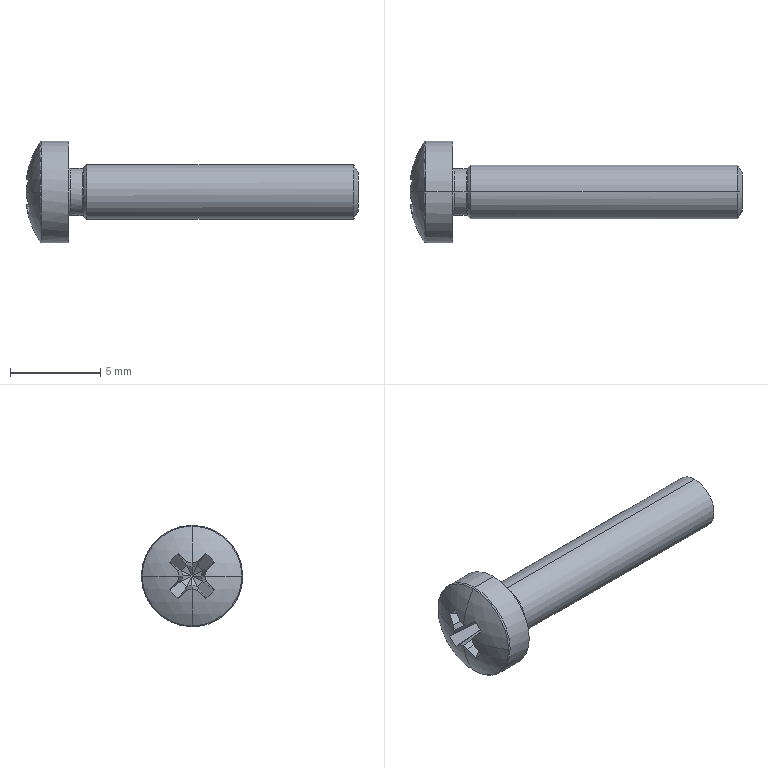Part | STEP file | 103000006242_M3×16 | 1 solid | 54 faces | box 18.351 x 5.6 x 5.6 mm | volume 155.702 mm3 | plane 34 | cylinder 6 | torus 6 | cone 4 | sphere 4 | commonest cylinder face diameters 2.598 x2 3 x2 5.6 x2
STEP:
#1=CARTESIAN_POINT('',(18.4,0.,1.067));
#2=VERTEX_POINT('',#1);
#3=CARTESIAN_POINT('',(18.4,0.,-1.067));
#4=VERTEX_POINT('',#3);
#5=CARTESIAN_POINT('',(18.4,0.,0.));
#6=DIRECTION('',(-1.,0.,0.));
#7=AXIS2_PLACEMENT_3D('',#5,#6,$);
#8=CIRCLE('',#7,1.067);
#9=EDGE_CURVE('',#2,#4,#8,.T.);
#10=ORIENTED_EDGE('',*,*,#9,.T.);
#11=CARTESIAN_POINT('',(18.153,0.,-1.5));
#12=VERTEX_POINT('',#11);
#13=CARTESIAN_POINT('',(-247947.644,0.,-434181.301));
#14=DIRECTION('',(-0.4959,0.,-0.8684));
#15=VECTOR('',#14,1.);
#16=LINE('',#13,#15);
#17=EDGE_CURVE('',#4,#12,#16,.T.);
#18=ORIENTED_EDGE('',*,*,#17,.T.);
#19=CARTESIAN_POINT('',(18.153,0.,1.5));
#20=VERTEX_POINT('',#19);
#21=CARTESIAN_POINT('',(18.153,0.,0.));
#22=DIRECTION('',(-1.,0.,0.));
#23=AXIS2_PLACEMENT_3D('',#21,#22,$);
#24=CIRCLE('',#23,1.5);
#25=EDGE_CURVE('',#20,#12,#24,.T.);
#26=ORIENTED_EDGE('',*,*,#25,.F.);
#27=CARTESIAN_POINT('',(-247947.644,0.,434181.301));
#28=DIRECTION('',(-0.4959,0.,0.8684));
#29=VECTOR('',#28,1.);
#30=LINE('',#27,#29);
#31=EDGE_CURVE('',#2,#20,#30,.T.);
#32=ORIENTED_EDGE('',*,*,#31,.F.);
#33=EDGE_LOOP('',(#10,#18,#26,#32));
#34=FACE_OUTER_BOUND('',#33,.T.);
#35=CARTESIAN_POINT('',(18.153,0.,0.));
#36=DIRECTION('',(-1.,0.,0.));
#37=DIRECTION('',(0.,0.,1.));
#38=AXIS2_PLACEMENT_3D('',#35,#36,#37);
#39=CONICAL_SURFACE('',#38,1.5,1.052);
#40=ADVANCED_FACE('',(#34),#39,.T.);
#41=ORIENTED_EDGE('',*,*,#9,.F.);
#42=CARTESIAN_POINT('',(18.4,0.,0.));
#43=DIRECTION('',(-1.,0.,0.));
#44=AXIS2_PLACEMENT_3D('',#42,#43,$);
#45=CIRCLE('',#44,1.067);
#46=EDGE_CURVE('',#4,#2,#45,.T.);
#47=ORIENTED_EDGE('',*,*,#46,.F.);
#48=EDGE_LOOP('',(#41,#47));
#49=FACE_OUTER_BOUND('',#48,.T.);
#50=CARTESIAN_POINT('',(18.4,0.,0.));
#51=DIRECTION('',(-1.,0.,0.));
#52=DIRECTION('',(0.,0.,1.));
#53=AXIS2_PLACEMENT_3D('',#50,#51,#52);
#54=PLANE('',#53);
#55=ADVANCED_FACE('',(#49),#54,.F.);
#56=ORIENTED_EDGE('',*,*,#17,.F.);
#57=ORIENTED_EDGE('',*,*,#46,.T.);
#58=ORIENTED_EDGE('',*,*,#31,.T.);
#59=CARTESIAN_POINT('',(18.153,0.,0.));
#60=DIRECTION('',(-1.,0.,0.));
#61=AXIS2_PLACEMENT_3D('',#59,#60,$);
#62=CIRCLE('',#61,1.5);
#63=EDGE_CURVE('',#12,#20,#62,.T.);
#64=ORIENTED_EDGE('',*,*,#63,.F.);
#65=EDGE_LOOP('',(#56,#57,#58,#64));
#66=FACE_OUTER_BOUND('',#65,.T.);
#67=CARTESIAN_POINT('',(18.153,0.,0.));
#68=DIRECTION('',(-1.,0.,0.));
#69=DIRECTION('',(0.,0.,-1.));
#70=AXIS2_PLACEMENT_3D('',#67,#68,#69);
#71=CONICAL_SURFACE('',#70,1.5,1.052);
#72=ADVANCED_FACE('',(#66),#71,.T.);
#73=ORIENTED_EDGE('',*,*,#25,.T.);
#74=CARTESIAN_POINT('',(3.4,0.,-1.5));
#75=VERTEX_POINT('',#74);
#76=CARTESIAN_POINT('',(-3.442,0.,-1.5));
#77=DIRECTION('',(-1.,0.,0.));
#78=VECTOR('',#77,1.);
#79=LINE('',#76,#78);
#80=EDGE_CURVE('',#12,#75,#79,.T.);
#81=ORIENTED_EDGE('',*,*,#80,.T.);
#82=CARTESIAN_POINT('',(3.4,0.,1.5));
#83=VERTEX_POINT('',#82);
#84=CARTESIAN_POINT('',(3.4,0.,0.));
#85=DIRECTION('',(-1.,0.,0.));
#86=AXIS2_PLACEMENT_3D('',#84,#85,$);
#87=CIRCLE('',#86,1.5);
#88=EDGE_CURVE('',#83,#75,#87,.T.);
#89=ORIENTED_EDGE('',*,*,#88,.F.);
#90=CARTESIAN_POINT('',(-3.442,0.,1.5));
#91=DIRECTION('',(-1.,0.,0.));
#92=VECTOR('',#91,1.);
#93=LINE('',#90,#92);
#94=EDGE_CURVE('',#20,#83,#93,.T.);
#95=ORIENTED_EDGE('',*,*,#94,.F.);
#96=EDGE_LOOP('',(#73,#81,#89,#95));
#97=FACE_OUTER_BOUND('',#96,.T.);
#98=CARTESIAN_POINT('',(-3.442,0.,0.));
#99=DIRECTION('',(-1.,0.,0.));
#100=DIRECTION('',(0.,0.,1.));
#101=AXIS2_PLACEMENT_3D('',#98,#99,#100);
#102=CYLINDRICAL_SURFACE('',#101,1.5);
#103=ADVANCED_FACE('',(#97),#102,.T.);
#104=ORIENTED_EDGE('',*,*,#80,.F.);
#105=ORIENTED_EDGE('',*,*,#63,.T.);
#106=ORIENTED_EDGE('',*,*,#94,.T.);
#107=CARTESIAN_POINT('',(3.4,0.,-1.5));
#108=CARTESIAN_POINT('',(3.4,-0.4712,-1.5));
#109=CARTESIAN_POINT('',(3.4,-0.9425,-1.315));
#110=CARTESIAN_POINT('',(3.4,-1.315,-0.9425));
#111=CARTESIAN_POINT('',(3.4,-1.685,0.));
#112=CARTESIAN_POINT('',(3.4,-1.315,0.9425));
#113=CARTESIAN_POINT('',(3.4,-0.9425,1.315));
#114=CARTESIAN_POINT('',(3.4,-0.4712,1.5));
#115=CARTESIAN_POINT('',(3.4,0.,1.5));
#116=B_SPLINE_CURVE_WITH_KNOTS('',5,(#107,#108,#109,#110,#111,#112,#113,#114,#115),.UNSPECIFIED.,.F.,.U.,(6,3,6),(-2.356,0.,2.356),.UNSPECIFIED.);
#117=EDGE_CURVE('',#75,#83,#116,.T.);
#118=ORIENTED_EDGE('',*,*,#117,.F.);
#119=EDGE_LOOP('',(#104,#105,#106,#118));
#120=FACE_OUTER_BOUND('',#119,.T.);
#121=CARTESIAN_POINT('',(-3.442,0.,0.));
#122=DIRECTION('',(-1.,0.,0.));
#123=DIRECTION('',(0.,0.,-1.));
#124=AXIS2_PLACEMENT_3D('',#121,#122,#123);
#125=CYLINDRICAL_SURFACE('',#124,1.5);
#126=ADVANCED_FACE('',(#120),#125,.T.);
#127=CARTESIAN_POINT('',(3.228,0.,-1.328));
#128=VERTEX_POINT('',#127);
#129=CARTESIAN_POINT('',(3.228,0.,1.328));
#130=VERTEX_POINT('',#129);
#131=CARTESIAN_POINT('',(3.228,0.,0.));
#132=DIRECTION('',(1.,0.,0.));
#133=AXIS2_PLACEMENT_3D('',#131,#132,$);
#134=CIRCLE('',#133,1.328);
#135=EDGE_CURVE('',#128,#130,#134,.T.);
#136=ORIENTED_EDGE('',*,*,#135,.T.);
#137=CARTESIAN_POINT('',(353556.041,0.,353554.141));
#138=DIRECTION('',(0.7071,0.,0.7071));
#139=VECTOR('',#138,1.);
#140=LINE('',#137,#139);
#141=EDGE_CURVE('',#130,#83,#140,.T.);
#142=ORIENTED_EDGE('',*,*,#141,.T.);
#143=ORIENTED_EDGE('',*,*,#88,.T.);
#144=CARTESIAN_POINT('',(353556.041,0.,-353554.141));
#145=DIRECTION('',(0.7071,0.,-0.7071));
#146=VECTOR('',#145,1.);
#147=LINE('',#144,#146);
#148=EDGE_CURVE('',#128,#75,#147,.T.);
#149=ORIENTED_EDGE('',*,*,#148,.F.);
#150=EDGE_LOOP('',(#136,#142,#143,#149));
#151=FACE_OUTER_BOUND('',#150,.T.);
#152=CARTESIAN_POINT('',(3.4,0.,0.));
#153=DIRECTION('',(1.,0.,0.));
#154=DIRECTION('',(0.,0.,-1.));
#155=AXIS2_PLACEMENT_3D('',#152,#153,#154);
#156=CONICAL_SURFACE('',#155,1.5,0.7854);
#157=ADVANCED_FACE('',(#151),#156,.T.);
#158=ORIENTED_EDGE('',*,*,#141,.F.);
#159=CARTESIAN_POINT('',(3.228,0.,0.));
#160=DIRECTION('',(1.,0.,0.));
#161=AXIS2_PLACEMENT_3D('',#159,#160,$);
#162=CIRCLE('',#161,1.328);
#163=EDGE_CURVE('',#130,#128,#162,.T.);
#164=ORIENTED_EDGE('',*,*,#163,.T.);
#165=ORIENTED_EDGE('',*,*,#148,.T.);
#166=ORIENTED_EDGE('',*,*,#117,.T.);
#167=EDGE_LOOP('',(#158,#164,#165,#166));
#168=FACE_OUTER_BOUND('',#167,.T.);
#169=CARTESIAN_POINT('',(3.4,0.,0.));
#170=DIRECTION('',(1.,0.,0.));
#171=DIRECTION('',(0.,0.,1.));
#172=AXIS2_PLACEMENT_3D('',#169,#170,#171);
#173=CONICAL_SURFACE('',#172,1.5,0.7854);
#174=ADVANCED_FACE('',(#168),#173,.T.);
#175=CARTESIAN_POINT('',(3.158,0.,-1.299));
#176=VERTEX_POINT('',#175);
#177=CARTESIAN_POINT('',(3.158,0.,-1.399));
#178=DIRECTION('',(0.,1.,0.));
#179=AXIS2_PLACEMENT_3D('',#177,#178,$);
#180=CIRCLE('',#179,0.1);
#181=EDGE_CURVE('',#176,#128,#180,.T.);
#182=ORIENTED_EDGE('',*,*,#181,.F.);
#183=CARTESIAN_POINT('',(3.158,0.,1.299));
#184=VERTEX_POINT('',#183);
#185=CARTESIAN_POINT('',(3.158,0.,0.));
#186=DIRECTION('',(-1.,0.,0.));
#187=AXIS2_PLACEMENT_3D('',#185,#186,$);
#188=CIRCLE('',#187,1.299);
#189=EDGE_CURVE('',#184,#176,#188,.T.);
#190=ORIENTED_EDGE('',*,*,#189,.F.);
#191=CARTESIAN_POINT('',(3.158,0.,1.399));
#192=DIRECTION('',(0.,-1.,0.));
#193=AXIS2_PLACEMENT_3D('',#191,#192,$);
#194=CIRCLE('',#193,0.1);
#195=EDGE_CURVE('',#184,#130,#194,.T.);
#196=ORIENTED_EDGE('',*,*,#195,.T.);
#197=ORIENTED_EDGE('',*,*,#135,.F.);
#198=EDGE_LOOP('',(#182,#190,#196,#197));
#199=FACE_OUTER_BOUND('',#198,.T.);
#200=CARTESIAN_POINT('',(3.158,0.,0.));
#201=DIRECTION('',(-1.,0.,0.));
#202=DIRECTION('',(0.,0.,1.));
#203=AXIS2_PLACEMENT_3D('',#200,#201,#202);
#204=TOROIDAL_SURFACE('',#203,1.399,0.1);
#205=ADVANCED_FACE('',(#199),#204,.F.);
#206=CARTESIAN_POINT('',(3.158,0.,0.));
#207=DIRECTION('',(-1.,0.,0.));
#208=AXIS2_PLACEMENT_3D('',#206,#207,$);
#209=CIRCLE('',#208,1.299);
#210=EDGE_CURVE('',#176,#184,#209,.T.);
#211=ORIENTED_EDGE('',*,*,#210,.F.);
#212=ORIENTED_EDGE('',*,*,#181,.T.);
#213=ORIENTED_EDGE('',*,*,#163,.F.);
#214=ORIENTED_EDGE('',*,*,#195,.F.);
#215=EDGE_LOOP('',(#211,#212,#213,#214));
#216=FACE_OUTER_BOUND('',#215,.T.);
#217=CARTESIAN_POINT('',(3.158,0.,0.));
#218=DIRECTION('',(-1.,0.,0.));
#219=DIRECTION('',(0.,0.,-1.));
#220=AXIS2_PLACEMENT_3D('',#217,#218,#219);
#221=TOROIDAL_SURFACE('',#220,1.399,0.1);
#222=ADVANCED_FACE('',(#216),#221,.F.);
#223=ORIENTED_EDGE('',*,*,#189,.T.);
#224=CARTESIAN_POINT('',(2.5,0.,-1.299));
#225=VERTEX_POINT('',#224);
#226=CARTESIAN_POINT('',(-3.442,0.,-1.299));
#227=DIRECTION('',(-1.,0.,0.));
#228=VECTOR('',#227,1.);
#229=LINE('',#226,#228);
#230=EDGE_CURVE('',#176,#225,#229,.T.);
#231=ORIENTED_EDGE('',*,*,#230,.T.);
#232=CARTESIAN_POINT('',(2.5,0.,1.299));
#233=VERTEX_POINT('',#232);
#234=CARTESIAN_POINT('',(2.5,0.,0.));
#235=DIRECTION('',(-1.,0.,0.));
#236=AXIS2_PLACEMENT_3D('',#234,#235,$);
#237=CIRCLE('',#236,1.299);
#238=EDGE_CURVE('',#225,#233,#237,.F.);
#239=ORIENTED_EDGE('',*,*,#238,.T.);
#240=CARTESIAN_POINT('',(-3.442,0.,1.299));
#241=DIRECTION('',(-1.,0.,0.));
#242=VECTOR('',#241,1.);
#243=LINE('',#240,#242);
#244=EDGE_CURVE('',#184,#233,#243,.T.);
#245=ORIENTED_EDGE('',*,*,#244,.F.);
#246=EDGE_LOOP('',(#223,#231,#239,#245));
#247=FACE_OUTER_BOUND('',#246,.T.);
#248=CARTESIAN_POINT('',(-3.442,0.,0.));
#249=DIRECTION('',(-1.,0.,0.));
#250=DIRECTION('',(0.,0.,1.));
#251=AXIS2_PLACEMENT_3D('',#248,#249,#250);
#252=CYLINDRICAL_SURFACE('',#251,1.299);
#253=ADVANCED_FACE('',(#247),#252,.T.);
#254=ORIENTED_EDGE('',*,*,#230,.F.);
#255=ORIENTED_EDGE('',*,*,#210,.T.);
#256=ORIENTED_EDGE('',*,*,#244,.T.);
#257=CARTESIAN_POINT('',(2.5,0.,1.299));
#258=CARTESIAN_POINT('',(2.5,-0.4081,1.299));
#259=CARTESIAN_POINT('',(2.5,-0.8162,1.139));
#260=CARTESIAN_POINT('',(2.5,-1.139,0.8162));
#261=CARTESIAN_POINT('',(2.5,-1.459,0.));
#262=CARTESIAN_POINT('',(2.5,-1.139,-0.8162));
#263=CARTESIAN_POINT('',(2.5,-0.8162,-1.139));
#264=CARTESIAN_POINT('',(2.5,-0.4081,-1.299));
#265=CARTESIAN_POINT('',(2.5,0.,-1.299));
#266=B_SPLINE_CURVE_WITH_KNOTS('',5,(#257,#258,#259,#260,#261,#262,#263,#264,#265),.UNSPECIFIED.,.F.,.U.,(6,3,6),(-2.04,0.,2.04),.UNSPECIFIED.);
#267=EDGE_CURVE('',#233,#225,#266,.T.);
#268=ORIENTED_EDGE('',*,*,#267,.T.);
#269=EDGE_LOOP('',(#254,#255,#256,#268));
#270=FACE_OUTER_BOUND('',#269,.T.);
#271=CARTESIAN_POINT('',(-3.442,0.,0.));
#272=DIRECTION('',(-1.,0.,0.));
#273=DIRECTION('',(0.,0.,-1.));
#274=AXIS2_PLACEMENT_3D('',#271,#272,#273);
#275=CYLINDRICAL_SURFACE('',#274,1.299);
#276=ADVANCED_FACE('',(#270),#275,.T.);
#277=CARTESIAN_POINT('',(2.4,0.,-1.399));
#278=VERTEX_POINT('',#277);
#279=CARTESIAN_POINT('',(2.5,0.,-1.399));
#280=DIRECTION('',(0.,1.,0.));
#281=AXIS2_PLACEMENT_3D('',#279,#280,$);
#282=CIRCLE('',#281,0.1);
#283=EDGE_CURVE('',#278,#225,#282,.T.);
#284=ORIENTED_EDGE('',*,*,#283,.F.);
#285=CARTESIAN_POINT('',(2.4,0.,1.399));
#286=VERTEX_POINT('',#285);
#287=CARTESIAN_POINT('',(2.4,0.,0.));
#288=DIRECTION('',(-1.,0.,0.));
#289=AXIS2_PLACEMENT_3D('',#287,#288,$);
#290=CIRCLE('',#289,1.399);
#291=EDGE_CURVE('',#286,#278,#290,.T.);
#292=ORIENTED_EDGE('',*,*,#291,.F.);
#293=CARTESIAN_POINT('',(2.5,0.,1.399));
#294=DIRECTION('',(0.,-1.,0.));
#295=AXIS2_PLACEMENT_3D('',#293,#294,$);
#296=CIRCLE('',#295,0.1);
#297=EDGE_CURVE('',#286,#233,#296,.T.);
#298=ORIENTED_EDGE('',*,*,#297,.T.);
#299=ORIENTED_EDGE('',*,*,#238,.F.);
#300=EDGE_LOOP('',(#284,#292,#298,#299));
#301=FACE_OUTER_BOUND('',#300,.T.);
#302=CARTESIAN_POINT('',(2.5,0.,0.));
#303=DIRECTION('',(-1.,0.,0.));
#304=DIRECTION('',(0.,0.,1.));
#305=AXIS2_PLACEMENT_3D('',#302,#303,#304);
#306=TOROIDAL_SURFACE('',#305,1.399,0.1);
#307=ADVANCED_FACE('',(#301),#306,.F.);
#308=CARTESIAN_POINT('',(2.4,0.,0.));
#309=DIRECTION('',(-1.,0.,0.));
#310=AXIS2_PLACEMENT_3D('',#308,#309,$);
#311=CIRCLE('',#310,1.399);
#312=EDGE_CURVE('',#278,#286,#311,.T.);
#313=ORIENTED_EDGE('',*,*,#312,.F.);
#314=ORIENTED_EDGE('',*,*,#283,.T.);
#315=ORIENTED_EDGE('',*,*,#267,.F.);
#316=ORIENTED_EDGE('',*,*,#297,.F.);
#317=EDGE_LOOP('',(#313,#314,#315,#316));
#318=FACE_OUTER_BOUND('',#317,.T.);
#319=CARTESIAN_POINT('',(2.5,0.,0.));
#320=DIRECTION('',(-1.,0.,0.));
#321=DIRECTION('',(0.,0.,-1.));
#322=AXIS2_PLACEMENT_3D('',#319,#320,#321);
#323=TOROIDAL_SURFACE('',#322,1.399,0.1);
#324=ADVANCED_FACE('',(#318),#323,.F.);
#325=CARTESIAN_POINT('',(2.4,0.,2.8));
#326=VERTEX_POINT('',#325);
#327=CARTESIAN_POINT('',(2.4,0.,-2.8));
#328=VERTEX_POINT('',#327);
#329=CARTESIAN_POINT('',(2.4,-0.000000001,0.));
#330=DIRECTION('',(-1.,0.,0.));
#331=AXIS2_PLACEMENT_3D('',#329,#330,$);
#332=CIRCLE('',#331,2.8);
#333=EDGE_CURVE('',#326,#328,#332,.T.);
#334=ORIENTED_EDGE('',*,*,#333,.F.);
#335=CARTESIAN_POINT('',(2.4,0.000000001,0.));
#336=DIRECTION('',(-1.,0.,0.));
#337=AXIS2_PLACEMENT_3D('',#335,#336,$);
#338=CIRCLE('',#337,2.8);
#339=EDGE_CURVE('',#328,#326,#338,.T.);
#340=ORIENTED_EDGE('',*,*,#339,.F.);
#341=EDGE_LOOP('',(#334,#340));
#342=FACE_OUTER_BOUND('',#341,.T.);
#343=ORIENTED_EDGE('',*,*,#291,.T.);
#344=ORIENTED_EDGE('',*,*,#312,.T.);
#345=EDGE_LOOP('',(#343,#344));
#346=FACE_BOUND('',#345,.T.);
#347=CARTESIAN_POINT('',(2.4,2.8,0.));
#348=DIRECTION('',(-1.,0.,0.));
#349=DIRECTION('',(0.,0.,1.));
#350=AXIS2_PLACEMENT_3D('',#347,#348,#349);
#351=PLANE('',#350);
#352=ADVANCED_FACE('',(#342,#346),#351,.F.);
#353=ORIENTED_EDGE('',*,*,#333,.T.);
#354=CARTESIAN_POINT('',(0.911,0.,-2.8));
#355=VERTEX_POINT('',#354);
#356=CARTESIAN_POINT('',(-3.442,0.,-2.8));
#357=DIRECTION('',(-1.,0.,0.));
#358=VECTOR('',#357,1.);
#359=LINE('',#356,#358);
#360=EDGE_CURVE('',#328,#355,#359,.T.);
#361=ORIENTED_EDGE('',*,*,#360,.T.);
#362=CARTESIAN_POINT('',(0.911,0.,2.8));
#363=VERTEX_POINT('',#362);
#364=CARTESIAN_POINT('',(0.911,0.,0.));
#365=DIRECTION('',(-1.,0.,0.));
#366=AXIS2_PLACEMENT_3D('',#364,#365,$);
#367=CIRCLE('',#366,2.8);
#368=EDGE_CURVE('',#355,#363,#367,.F.);
#369=ORIENTED_EDGE('',*,*,#368,.T.);
#370=CARTESIAN_POINT('',(-3.442,0.,2.8));
#371=DIRECTION('',(-1.,0.,0.));
#372=VECTOR('',#371,1.);
#373=LINE('',#370,#372);
#374=EDGE_CURVE('',#326,#363,#373,.T.);
#375=ORIENTED_EDGE('',*,*,#374,.F.);
#376=EDGE_LOOP('',(#353,#361,#369,#375));
#377=FACE_OUTER_BOUND('',#376,.T.);
#378=CARTESIAN_POINT('',(-3.442,0.,0.));
#379=DIRECTION('',(-1.,0.,0.));
#380=DIRECTION('',(0.,0.,1.));
#381=AXIS2_PLACEMENT_3D('',#378,#379,#380);
#382=CYLINDRICAL_SURFACE('',#381,2.8);
#383=ADVANCED_FACE('',(#377),#382,.T.);
#384=ORIENTED_EDGE('',*,*,#360,.F.);
#385=ORIENTED_EDGE('',*,*,#339,.T.);
#386=ORIENTED_EDGE('',*,*,#374,.T.);
#387=CARTESIAN_POINT('',(0.911,0.,2.8));
#388=CARTESIAN_POINT('',(0.911,-0.8796,2.8));
#389=CARTESIAN_POINT('',(0.911,-1.759,2.455));
#390=CARTESIAN_POINT('',(0.911,-2.455,1.759));
#391=CARTESIAN_POINT('',(0.911,-3.145,0.));
#392=CARTESIAN_POINT('',(0.911,-2.455,-1.759));
#393=CARTESIAN_POINT('',(0.911,-1.759,-2.455));
#394=CARTESIAN_POINT('',(0.911,-0.8796,-2.8));
#395=CARTESIAN_POINT('',(0.911,0.,-2.8));
#396=B_SPLINE_CURVE_WITH_KNOTS('',5,(#387,#388,#389,#390,#391,#392,#393,#394,#395),.UNSPECIFIED.,.F.,.U.,(6,3,6),(-4.398,0.,4.398),.UNSPECIFIED.);
#397=EDGE_CURVE('',#363,#355,#396,.T.);
#398=ORIENTED_EDGE('',*,*,#397,.T.);
#399=EDGE_LOOP('',(#384,#385,#386,#398));
#400=FACE_OUTER_BOUND('',#399,.T.);
#401=CARTESIAN_POINT('',(-3.442,0.,0.));
#402=DIRECTION('',(-1.,0.,0.));
#403=DIRECTION('',(0.,0.,-1.));
#404=AXIS2_PLACEMENT_3D('',#401,#402,#403);
#405=CYLINDRICAL_SURFACE('',#404,2.8);
#406=ADVANCED_FACE('',(#400),#405,.T.);
#407=CARTESIAN_POINT('',(0.8275,0.,2.755));
#408=VERTEX_POINT('',#407);
#409=CARTESIAN_POINT('',(0.8275,2.755,0.));
#410=VERTEX_POINT('',#409);
#411=CARTESIAN_POINT('',(0.8275,0.,0.));
#412=DIRECTION('',(1.,0.,0.));
#413=AXIS2_PLACEMENT_3D('',#411,#412,$);
#414=CIRCLE('',#413,2.755);
#415=EDGE_CURVE('',#408,#410,#414,.F.);
#416=ORIENTED_EDGE('',*,*,#415,.F.);
#417=CARTESIAN_POINT('',(0.911,0.,2.7));
#418=DIRECTION('',(0.,1.,0.));
#419=AXIS2_PLACEMENT_3D('',#417,#418,$);
#420=CIRCLE('',#419,0.1);
#421=EDGE_CURVE('',#408,#363,#420,.T.);
#422=ORIENTED_EDGE('',*,*,#421,.T.);
#423=ORIENTED_EDGE('',*,*,#368,.F.);
#424=CARTESIAN_POINT('',(0.8275,0.,-2.755));
#425=VERTEX_POINT('',#424);
#426=CARTESIAN_POINT('',(0.911,0.,-2.7));
#427=DIRECTION('',(0.,-1.,0.));
#428=AXIS2_PLACEMENT_3D('',#426,#427,$);
#429=CIRCLE('',#428,0.1);
#430=EDGE_CURVE('',#425,#355,#429,.T.);
#431=ORIENTED_EDGE('',*,*,#430,.F.);
#432=CARTESIAN_POINT('',(0.8275,0.,0.));
#433=DIRECTION('',(1.,0.,0.));
#434=AXIS2_PLACEMENT_3D('',#432,#433,$);
#435=CIRCLE('',#434,2.755);
#436=EDGE_CURVE('',#410,#425,#435,.F.);
#437=ORIENTED_EDGE('',*,*,#436,.F.);
#438=EDGE_LOOP('',(#416,#422,#423,#431,#437));
#439=FACE_OUTER_BOUND('',#438,.T.);
#440=CARTESIAN_POINT('',(0.911,0.,0.));
#441=DIRECTION('',(1.,0.,0.));
#442=DIRECTION('',(0.,0.,-1.));
#443=AXIS2_PLACEMENT_3D('',#440,#441,#442);
#444=TOROIDAL_SURFACE('',#443,2.7,0.1);
#445=ADVANCED_FACE('',(#439),#444,.T.);
#446=ORIENTED_EDGE('',*,*,#421,.F.);
#447=CARTESIAN_POINT('',(0.8275,-2.755,0.));
#448=VERTEX_POINT('',#447);
#449=CARTESIAN_POINT('',(0.8275,0.,0.));
#450=DIRECTION('',(1.,0.,0.));
#451=AXIS2_PLACEMENT_3D('',#449,#450,$);
#452=CIRCLE('',#451,2.755);
#453=EDGE_CURVE('',#448,#408,#452,.F.);
#454=ORIENTED_EDGE('',*,*,#453,.F.);
#455=CARTESIAN_POINT('',(0.8275,0.,0.));
#456=DIRECTION('',(1.,0.,0.));
#457=AXIS2_PLACEMENT_3D('',#455,#456,$);
#458=CIRCLE('',#457,2.755);
#459=EDGE_CURVE('',#425,#448,#458,.F.);
#460=ORIENTED_EDGE('',*,*,#459,.F.);
#461=ORIENTED_EDGE('',*,*,#430,.T.);
#462=ORIENTED_EDGE('',*,*,#397,.F.);
#463=EDGE_LOOP('',(#446,#454,#460,#461,#462));
#464=FACE_OUTER_BOUND('',#463,.T.);
#465=CARTESIAN_POINT('',(0.911,0.,0.));
#466=DIRECTION('',(1.,0.,0.));
#467=DIRECTION('',(0.,0.,1.));
#468=AXIS2_PLACEMENT_3D('',#465,#466,#467);
#469=TOROIDAL_SURFACE('',#468,2.7,0.1);
#470=ADVANCED_FACE('',(#464),#469,.T.);
#471=CARTESIAN_POINT('',(0.04924,0.,0.7));
#472=VERTEX_POINT('',#471);
#473=CARTESIAN_POINT('',(5.,0.,0.));
#474=DIRECTION('',(0.,-1.,0.));
#475=AXIS2_PLACEMENT_3D('',#473,#474,$);
#476=CIRCLE('',#475,5.);
#477=EDGE_CURVE('',#408,#472,#476,.T.);
#478=ORIENTED_EDGE('',*,*,#477,.F.);
#479=ORIENTED_EDGE('',*,*,#415,.T.);
#480=CARTESIAN_POINT('',(0.04924,0.7,0.));
#481=VERTEX_POINT('',#480);
#482=CARTESIAN_POINT('',(5.,0.,0.));
#483=DIRECTION('',(0.,0.,-1.));
#484=AXIS2_PLACEMENT_3D('',#482,#483,$);
#485=CIRCLE('',#484,5.);
#486=EDGE_CURVE('',#410,#481,#485,.F.);
#487=ORIENTED_EDGE('',*,*,#486,.T.);
#488=CARTESIAN_POINT('',(0.0753,0.8113,0.2985));
#489=VERTEX_POINT('',#488);
#490=CARTESIAN_POINT('',(0.04924,0.7,0.));
#491=CARTESIAN_POINT('',(0.05455,0.7375,0.09958));
#492=CARTESIAN_POINT('',(0.06324,0.7747,0.1991));
#493=CARTESIAN_POINT('',(0.0753,0.8113,0.2985));
#494=B_SPLINE_CURVE_WITH_KNOTS('',3,(#490,#491,#492,#493),.UNSPECIFIED.,.F.,.U.,(4,4),(0.,0.4521),.UNSPECIFIED.);
#495=EDGE_CURVE('',#481,#489,#494,.T.);
#496=ORIENTED_EDGE('',*,*,#495,.T.);
#497=CARTESIAN_POINT('',(0.2189,1.246,0.7669));
#498=VERTEX_POINT('',#497);
#499=CARTESIAN_POINT('',(0.0753,0.8113,0.2985));
#500=CARTESIAN_POINT('',(0.1092,0.9593,0.4559));
#501=CARTESIAN_POINT('',(0.1573,1.105,0.6126));
#502=CARTESIAN_POINT('',(0.2189,1.246,0.7669));
#503=B_SPLINE_CURVE_WITH_KNOTS('',3,(#499,#500,#501,#502),.UNSPECIFIED.,.F.,.U.,(4,4),(0.,0.9283),.UNSPECIFIED.);
#504=EDGE_CURVE('',#489,#498,#503,.T.);
#505=ORIENTED_EDGE('',*,*,#504,.T.);
#506=CARTESIAN_POINT('',(0.2189,0.7669,1.246));
#507=VERTEX_POINT('',#506);
#508=CARTESIAN_POINT('',(0.2189,0.7669,1.246));
#509=CARTESIAN_POINT('',(0.205,0.9307,1.092));
#510=CARTESIAN_POINT('',(0.2049,1.091,0.9316));
#511=CARTESIAN_POINT('',(0.2189,1.246,0.7669));
#512=B_SPLINE_CURVE_WITH_KNOTS('',3,(#508,#509,#510,#511),.UNSPECIFIED.,.F.,.U.,(4,4),(0.,0.9641),.UNSPECIFIED.);
#513=EDGE_CURVE('',#507,#498,#512,.T.);
#514=ORIENTED_EDGE('',*,*,#513,.F.);
#515=CARTESIAN_POINT('',(0.0753,0.2985,0.8113));
#516=VERTEX_POINT('',#515);
#517=CARTESIAN_POINT('',(0.2189,0.7669,1.246));
#518=CARTESIAN_POINT('',(0.1574,0.6128,1.105));
#519=CARTESIAN_POINT('',(0.1093,0.4562,0.9595));
#520=CARTESIAN_POINT('',(0.0753,0.2985,0.8113));
#521=B_SPLINE_CURVE_WITH_KNOTS('',3,(#517,#518,#519,#520),.UNSPECIFIED.,.F.,.U.,(4,4),(0.,0.9325),.UNSPECIFIED.);
#522=EDGE_CURVE('',#507,#516,#521,.T.);
#523=ORIENTED_EDGE('',*,*,#522,.T.);
#524=CARTESIAN_POINT('',(0.0753,0.2985,0.8113));
#525=CARTESIAN_POINT('',(0.06325,0.1992,0.7747));
#526=CARTESIAN_POINT('',(0.05455,0.09965,0.7376));
#527=CARTESIAN_POINT('',(0.04924,0.,0.7));
#528=B_SPLINE_CURVE_WITH_KNOTS('',3,(#524,#525,#526,#527),.UNSPECIFIED.,.F.,.U.,(4,4),(0.,0.4544),.UNSPECIFIED.);
#529=EDGE_CURVE('',#516,#472,#528,.T.);
#530=ORIENTED_EDGE('',*,*,#529,.T.);
#531=EDGE_LOOP('',(#478,#479,#487,#496,#505,#514,#523,#530));
#532=FACE_OUTER_BOUND('',#531,.T.);
#533=CARTESIAN_POINT('',(5.,0.,0.));
#534=DIRECTION('',(0.,0.,-1.));
#535=DIRECTION('',(-1.,0.,0.));
#536=AXIS2_PLACEMENT_3D('',#533,#534,#535);
#537=SPHERICAL_SURFACE('',#536,5.);
#538=ADVANCED_FACE('',(#532),#537,.T.);
#539=CARTESIAN_POINT('',(0.04924,0.,-0.7));
#540=VERTEX_POINT('',#539);
#541=CARTESIAN_POINT('',(5.,0.,0.));
#542=DIRECTION('',(0.,-1.,0.));
#543=AXIS2_PLACEMENT_3D('',#541,#542,$);
#544=CIRCLE('',#543,5.);
#545=EDGE_CURVE('',#540,#425,#544,.T.);
#546=ORIENTED_EDGE('',*,*,#545,.F.);
#547=CARTESIAN_POINT('',(0.0753,0.2985,-0.8113));
#548=VERTEX_POINT('',#547);
#549=CARTESIAN_POINT('',(0.04924,0.,-0.7));
#550=CARTESIAN_POINT('',(0.05455,0.09965,-0.7376));
#551=CARTESIAN_POINT('',(0.06325,0.1992,-0.7747));
#552=CARTESIAN_POINT('',(0.0753,0.2985,-0.8113));
#553=B_SPLINE_CURVE_WITH_KNOTS('',3,(#549,#550,#551,#552),.UNSPECIFIED.,.F.,.U.,(4,4),(0.,0.4544),.UNSPECIFIED.);
#554=EDGE_CURVE('',#540,#548,#553,.T.);
#555=ORIENTED_EDGE('',*,*,#554,.T.);
#556=CARTESIAN_POINT('',(0.2189,0.7669,-1.246));
#557=VERTEX_POINT('',#556);
#558=CARTESIAN_POINT('',(0.0753,0.2985,-0.8113));
#559=CARTESIAN_POINT('',(0.1093,0.4562,-0.9595));
#560=CARTESIAN_POINT('',(0.1574,0.6128,-1.105));
#561=CARTESIAN_POINT('',(0.2189,0.7669,-1.246));
#562=B_SPLINE_CURVE_WITH_KNOTS('',3,(#558,#559,#560,#561),.UNSPECIFIED.,.F.,.U.,(4,4),(0.,0.9325),.UNSPECIFIED.);
#563=EDGE_CURVE('',#548,#557,#562,.T.);
#564=ORIENTED_EDGE('',*,*,#563,.T.);
#565=CARTESIAN_POINT('',(0.2189,1.246,-0.7669));
#566=VERTEX_POINT('',#565);
#567=CARTESIAN_POINT('',(0.2189,1.246,-0.7669));
#568=CARTESIAN_POINT('',(0.2049,1.091,-0.9316));
#569=CARTESIAN_POINT('',(0.205,0.9307,-1.092));
#570=CARTESIAN_POINT('',(0.2189,0.7669,-1.246));
#571=B_SPLINE_CURVE_WITH_KNOTS('',3,(#567,#568,#569,#570),.UNSPECIFIED.,.F.,.U.,(4,4),(0.,0.9641),.UNSPECIFIED.);
#572=EDGE_CURVE('',#566,#557,#571,.T.);
#573=ORIENTED_EDGE('',*,*,#572,.F.);
#574=CARTESIAN_POINT('',(0.0753,0.8113,-0.2985));
#575=VERTEX_POINT('',#574);
#576=CARTESIAN_POINT('',(0.2189,1.246,-0.7669));
#577=CARTESIAN_POINT('',(0.1573,1.105,-0.6126));
#578=CARTESIAN_POINT('',(0.1092,0.9593,-0.4559));
#579=CARTESIAN_POINT('',(0.0753,0.8113,-0.2985));
#580=B_SPLINE_CURVE_WITH_KNOTS('',3,(#576,#577,#578,#579),.UNSPECIFIED.,.F.,.U.,(4,4),(0.,0.9283),.UNSPECIFIED.);
#581=EDGE_CURVE('',#566,#575,#580,.T.);
#582=ORIENTED_EDGE('',*,*,#581,.T.);
#583=CARTESIAN_POINT('',(0.0753,0.8113,-0.2985));
#584=CARTESIAN_POINT('',(0.06324,0.7747,-0.1991));
#585=CARTESIAN_POINT('',(0.05455,0.7375,-0.09958));
#586=CARTESIAN_POINT('',(0.04924,0.7,0.));
#587=B_SPLINE_CURVE_WITH_KNOTS('',3,(#583,#584,#585,#586),.UNSPECIFIED.,.F.,.U.,(4,4),(0.,0.4521),.UNSPECIFIED.);
#588=EDGE_CURVE('',#575,#481,#587,.T.);
#589=ORIENTED_EDGE('',*,*,#588,.T.);
#590=ORIENTED_EDGE('',*,*,#486,.F.);
#591=ORIENTED_EDGE('',*,*,#436,.T.);
#592=EDGE_LOOP('',(#546,#555,#564,#573,#582,#589,#590,#591));
#593=FACE_OUTER_BOUND('',#592,.T.);
#594=CARTESIAN_POINT('',(5.,0.,0.));
#595=DIRECTION('',(0.,0.,-1.));
#596=DIRECTION('',(-1.,0.,0.));
#597=AXIS2_PLACEMENT_3D('',#594,#595,#596);
#598=SPHERICAL_SURFACE('',#597,5.);
#599=ADVANCED_FACE('',(#593),#598,.T.);
#600=ORIENTED_EDGE('',*,*,#477,.T.);
#601=CARTESIAN_POINT('',(0.0753,-0.2985,0.8113));
#602=VERTEX_POINT('',#601);
#603=CARTESIAN_POINT('',(0.04924,0.,0.7));
#604=CARTESIAN_POINT('',(0.05455,-0.09965,0.7376));
#605=CARTESIAN_POINT('',(0.06325,-0.1992,0.7747));
#606=CARTESIAN_POINT('',(0.0753,-0.2985,0.8113));
#607=B_SPLINE_CURVE_WITH_KNOTS('',3,(#603,#604,#605,#606),.UNSPECIFIED.,.F.,.U.,(4,4),(0.,0.4544),.UNSPECIFIED.);
#608=EDGE_CURVE('',#472,#602,#607,.T.);
#609=ORIENTED_EDGE('',*,*,#608,.T.);
#610=CARTESIAN_POINT('',(0.2189,-0.7669,1.246));
#611=VERTEX_POINT('',#610);
#612=CARTESIAN_POINT('',(0.0753,-0.2985,0.8113));
#613=CARTESIAN_POINT('',(0.1093,-0.4562,0.9595));
#614=CARTESIAN_POINT('',(0.1574,-0.6128,1.105));
#615=CARTESIAN_POINT('',(0.2189,-0.7669,1.246));
#616=B_SPLINE_CURVE_WITH_KNOTS('',3,(#612,#613,#614,#615),.UNSPECIFIED.,.F.,.U.,(4,4),(0.,0.9325),.UNSPECIFIED.);
#617=EDGE_CURVE('',#602,#611,#616,.T.);
#618=ORIENTED_EDGE('',*,*,#617,.T.);
#619=CARTESIAN_POINT('',(0.2189,-1.246,0.7669));
#620=VERTEX_POINT('',#619);
#621=CARTESIAN_POINT('',(0.2189,-1.246,0.7669));
#622=CARTESIAN_POINT('',(0.2049,-1.091,0.9316));
#623=CARTESIAN_POINT('',(0.205,-0.9307,1.092));
#624=CARTESIAN_POINT('',(0.2189,-0.7669,1.246));
#625=B_SPLINE_CURVE_WITH_KNOTS('',3,(#621,#622,#623,#624),.UNSPECIFIED.,.F.,.U.,(4,4),(0.,0.9641),.UNSPECIFIED.);
#626=EDGE_CURVE('',#620,#611,#625,.T.);
#627=ORIENTED_EDGE('',*,*,#626,.F.);
#628=CARTESIAN_POINT('',(0.0753,-0.8113,0.2985));
#629=VERTEX_POINT('',#628);
#630=CARTESIAN_POINT('',(0.2189,-1.246,0.7669));
#631=CARTESIAN_POINT('',(0.1573,-1.105,0.6126));
#632=CARTESIAN_POINT('',(0.1092,-0.9593,0.4559));
#633=CARTESIAN_POINT('',(0.0753,-0.8113,0.2985));
#634=B_SPLINE_CURVE_WITH_KNOTS('',3,(#630,#631,#632,#633),.UNSPECIFIED.,.F.,.U.,(4,4),(0.,0.9283),.UNSPECIFIED.);
#635=EDGE_CURVE('',#620,#629,#634,.T.);
#636=ORIENTED_EDGE('',*,*,#635,.T.);
#637=CARTESIAN_POINT('',(0.04924,-0.7,0.));
#638=VERTEX_POINT('',#637);
#639=CARTESIAN_POINT('',(0.0753,-0.8113,0.2985));
#640=CARTESIAN_POINT('',(0.06324,-0.7747,0.1991));
#641=CARTESIAN_POINT('',(0.05455,-0.7375,0.09958));
#642=CARTESIAN_POINT('',(0.04924,-0.7,0.));
#643=B_SPLINE_CURVE_WITH_KNOTS('',3,(#639,#640,#641,#642),.UNSPECIFIED.,.F.,.U.,(4,4),(0.,0.4521),.UNSPECIFIED.);
#644=EDGE_CURVE('',#629,#638,#643,.T.);
#645=ORIENTED_EDGE('',*,*,#644,.T.);
#646=CARTESIAN_POINT('',(5.,0.,0.));
#647=DIRECTION('',(0.,0.,-1.));
#648=AXIS2_PLACEMENT_3D('',#646,#647,$);
#649=CIRCLE('',#648,5.);
#650=EDGE_CURVE('',#448,#638,#649,.T.);
#651=ORIENTED_EDGE('',*,*,#650,.F.);
#652=ORIENTED_EDGE('',*,*,#453,.T.);
#653=EDGE_LOOP('',(#600,#609,#618,#627,#636,#645,#651,#652));
#654=FACE_OUTER_BOUND('',#653,.T.);
#655=CARTESIAN_POINT('',(5.,0.,0.));
#656=DIRECTION('',(0.,0.,-1.));
#657=DIRECTION('',(0.,-1.,0.));
#658=AXIS2_PLACEMENT_3D('',#655,#656,#657);
#659=SPHERICAL_SURFACE('',#658,5.);
#660=ADVANCED_FACE('',(#654),#659,.T.);
#661=ORIENTED_EDGE('',*,*,#545,.T.);
#662=ORIENTED_EDGE('',*,*,#459,.T.);
#663=ORIENTED_EDGE('',*,*,#650,.T.);
#664=CARTESIAN_POINT('',(0.0753,-0.8113,-0.2985));
#665=VERTEX_POINT('',#664);
#666=CARTESIAN_POINT('',(0.04924,-0.7,0.));
#667=CARTESIAN_POINT('',(0.05455,-0.7375,-0.09958));
#668=CARTESIAN_POINT('',(0.06324,-0.7747,-0.1991));
#669=CARTESIAN_POINT('',(0.0753,-0.8113,-0.2985));
#670=B_SPLINE_CURVE_WITH_KNOTS('',3,(#666,#667,#668,#669),.UNSPECIFIED.,.F.,.U.,(4,4),(0.,0.4521),.UNSPECIFIED.);
#671=EDGE_CURVE('',#638,#665,#670,.T.);
#672=ORIENTED_EDGE('',*,*,#671,.T.);
#673=CARTESIAN_POINT('',(0.2189,-1.246,-0.7669));
#674=VERTEX_POINT('',#673);
#675=CARTESIAN_POINT('',(0.0753,-0.8113,-0.2985));
#676=CARTESIAN_POINT('',(0.1092,-0.9593,-0.4559));
#677=CARTESIAN_POINT('',(0.1573,-1.105,-0.6126));
#678=CARTESIAN_POINT('',(0.2189,-1.246,-0.7669));
#679=B_SPLINE_CURVE_WITH_KNOTS('',3,(#675,#676,#677,#678),.UNSPECIFIED.,.F.,.U.,(4,4),(0.,0.9283),.UNSPECIFIED.);
#680=EDGE_CURVE('',#665,#674,#679,.T.);
#681=ORIENTED_EDGE('',*,*,#680,.T.);
#682=CARTESIAN_POINT('',(0.2189,-0.7669,-1.246));
#683=VERTEX_POINT('',#682);
#684=CARTESIAN_POINT('',(0.2189,-0.7669,-1.246));
#685=CARTESIAN_POINT('',(0.205,-0.9307,-1.092));
#686=CARTESIAN_POINT('',(0.2049,-1.091,-0.9316));
#687=CARTESIAN_POINT('',(0.2189,-1.246,-0.7669));
#688=B_SPLINE_CURVE_WITH_KNOTS('',3,(#684,#685,#686,#687),.UNSPECIFIED.,.F.,.U.,(4,4),(0.,0.9641),.UNSPECIFIED.);
#689=EDGE_CURVE('',#683,#674,#688,.T.);
#690=ORIENTED_EDGE('',*,*,#689,.F.);
#691=CARTESIAN_POINT('',(0.0753,-0.2985,-0.8113));
#692=VERTEX_POINT('',#691);
#693=CARTESIAN_POINT('',(0.2189,-0.7669,-1.246));
#694=CARTESIAN_POINT('',(0.1574,-0.6128,-1.105));
#695=CARTESIAN_POINT('',(0.1093,-0.4562,-0.9595));
#696=CARTESIAN_POINT('',(0.0753,-0.2985,-0.8113));
#697=B_SPLINE_CURVE_WITH_KNOTS('',3,(#693,#694,#695,#696),.UNSPECIFIED.,.F.,.U.,(4,4),(0.,0.9325),.UNSPECIFIED.);
#698=EDGE_CURVE('',#683,#692,#697,.T.);
#699=ORIENTED_EDGE('',*,*,#698,.T.);
#700=CARTESIAN_POINT('',(0.0753,-0.2985,-0.8113));
#701=CARTESIAN_POINT('',(0.06325,-0.1992,-0.7747));
#702=CARTESIAN_POINT('',(0.05455,-0.09965,-0.7376));
#703=CARTESIAN_POINT('',(0.04924,0.,-0.7));
#704=B_SPLINE_CURVE_WITH_KNOTS('',3,(#700,#701,#702,#703),.UNSPECIFIED.,.F.,.U.,(4,4),(0.,0.4544),.UNSPECIFIED.);
#705=EDGE_CURVE('',#692,#540,#704,.T.);
#706=ORIENTED_EDGE('',*,*,#705,.T.);
#707=EDGE_LOOP('',(#661,#662,#663,#672,#681,#690,#699,#706));
#708=FACE_OUTER_BOUND('',#707,.T.);
#709=CARTESIAN_POINT('',(5.,0.,0.));
#710=DIRECTION('',(0.,0.,-1.));
#711=DIRECTION('',(0.,-1.,0.));
#712=AXIS2_PLACEMENT_3D('',#709,#710,#711);
#713=SPHERICAL_SURFACE('',#712,5.);
#714=ADVANCED_FACE('',(#708),#713,.T.);
#715=CARTESIAN_POINT('',(1.8,0.485,0.000000001));
#716=VERTEX_POINT('',#715);
#717=CARTESIAN_POINT('',(0.9246,0.5925,0.));
#718=DIRECTION('',(0.9925,-0.1219,-0.000000001));
#719=VECTOR('',#718,1.);
#720=LINE('',#717,#719);
#721=EDGE_CURVE('',#481,#716,#720,.T.);
#722=ORIENTED_EDGE('',*,*,#721,.T.);
#723=CARTESIAN_POINT('',(1.8,0.5996,0.2985));
#724=VERTEX_POINT('',#723);
#725=CARTESIAN_POINT('',(1.8,0.5423,0.1492));
#726=DIRECTION('',(0.,0.3584,0.9336));
#727=VECTOR('',#726,1.);
#728=LINE('',#725,#727);
#729=EDGE_CURVE('',#716,#724,#728,.T.);
#730=ORIENTED_EDGE('',*,*,#729,.T.);
#731=CARTESIAN_POINT('',(0.9377,0.7055,0.2985));
#732=DIRECTION('',(0.9925,-0.1219,0.));
#733=VECTOR('',#732,1.);
#734=LINE('',#731,#733);
#735=EDGE_CURVE('',#489,#724,#734,.T.);
#736=ORIENTED_EDGE('',*,*,#735,.F.);
#737=ORIENTED_EDGE('',*,*,#495,.F.);
#738=EDGE_LOOP('',(#722,#730,#736,#737));
#739=FACE_OUTER_BOUND('',#738,.T.);
#740=CARTESIAN_POINT('',(0.,0.706,0.));
#741=DIRECTION('',(0.1139,0.9275,-0.356));
#742=DIRECTION('',(0.,0.3584,0.9336));
#743=AXIS2_PLACEMENT_3D('',#740,#741,#742);
#744=PLANE('',#743);
#745=ADVANCED_FACE('',(#739),#744,.F.);
#746=ORIENTED_EDGE('',*,*,#735,.T.);
#747=CARTESIAN_POINT('',(1.009,0.9228,0.5327));
#748=DIRECTION('',(0.8927,-0.365,-0.2644));
#749=VECTOR('',#748,1.);
#750=LINE('',#747,#749);
#751=EDGE_CURVE('',#498,#724,#750,.T.);
#752=ORIENTED_EDGE('',*,*,#751,.F.);
#753=ORIENTED_EDGE('',*,*,#504,.F.);
#754=EDGE_LOOP('',(#746,#752,#753));
#755=FACE_OUTER_BOUND('',#754,.T.);
#756=CARTESIAN_POINT('',(0.,0.8206,0.2985));
#757=DIRECTION('',(0.08798,0.7166,-0.692));
#758=DIRECTION('',(0.,0.6947,0.7193));
#759=AXIS2_PLACEMENT_3D('',#756,#757,#758);
#760=PLANE('',#759);
#761=ADVANCED_FACE('',(#755),#760,.F.);
#762=ORIENTED_EDGE('',*,*,#513,.T.);
#763=ORIENTED_EDGE('',*,*,#751,.T.);
#764=CARTESIAN_POINT('',(1.8,0.2985,0.5996));
#765=VERTEX_POINT('',#764);
#766=CARTESIAN_POINT('',(1.8,0.449,0.449));
#767=DIRECTION('',(0.,-0.7071,0.7071));
#768=VECTOR('',#767,1.);
#769=LINE('',#766,#768);
#770=EDGE_CURVE('',#724,#765,#769,.T.);
#771=ORIENTED_EDGE('',*,*,#770,.T.);
#772=CARTESIAN_POINT('',(1.009,0.5327,0.9228));
#773=DIRECTION('',(-0.8927,0.2644,0.365));
#774=VECTOR('',#773,1.);
#775=LINE('',#772,#774);
#776=EDGE_CURVE('',#765,#507,#775,.T.);
#777=ORIENTED_EDGE('',*,*,#776,.T.);
#778=EDGE_LOOP('',(#762,#763,#771,#777));
#779=FACE_OUTER_BOUND('',#778,.T.);
#780=CARTESIAN_POINT('',(1.8,0.2985,0.5996));
#781=DIRECTION('',(-0.4462,-0.6328,-0.6328));
#782=DIRECTION('',(0.,0.7071,-0.7071));
#783=AXIS2_PLACEMENT_3D('',#780,#781,#782);
#784=PLANE('',#783);
#785=ADVANCED_FACE('',(#779),#784,.T.);
#786=ORIENTED_EDGE('',*,*,#776,.F.);
#787=CARTESIAN_POINT('',(0.9377,0.2985,0.7055));
#788=DIRECTION('',(0.9925,0.,-0.1219));
#789=VECTOR('',#788,1.);
#790=LINE('',#787,#789);
#791=EDGE_CURVE('',#516,#765,#790,.T.);
#792=ORIENTED_EDGE('',*,*,#791,.F.);
#793=ORIENTED_EDGE('',*,*,#522,.F.);
#794=EDGE_LOOP('',(#786,#792,#793));
#795=FACE_OUTER_BOUND('',#794,.T.);
#796=CARTESIAN_POINT('',(0.,0.8317,1.336));
#797=DIRECTION('',(0.08798,-0.692,0.7166));
#798=DIRECTION('',(0.,-0.7193,-0.6947));
#799=AXIS2_PLACEMENT_3D('',#796,#797,#798);
#800=PLANE('',#799);
#801=ADVANCED_FACE('',(#795),#800,.F.);
#802=ORIENTED_EDGE('',*,*,#791,.T.);
#803=CARTESIAN_POINT('',(1.8,-0.000000001,0.485));
#804=VERTEX_POINT('',#803);
#805=CARTESIAN_POINT('',(1.8,0.1492,0.5423));
#806=DIRECTION('',(0.,-0.9336,-0.3584));
#807=VECTOR('',#806,1.);
#808=LINE('',#805,#807);
#809=EDGE_CURVE('',#765,#804,#808,.T.);
#810=ORIENTED_EDGE('',*,*,#809,.T.);
#811=CARTESIAN_POINT('',(0.9246,0.,0.5925));
#812=DIRECTION('',(0.9925,-0.000000001,-0.1219));
#813=VECTOR('',#812,1.);
#814=LINE('',#811,#813);
#815=EDGE_CURVE('',#472,#804,#814,.T.);
#816=ORIENTED_EDGE('',*,*,#815,.F.);
#817=ORIENTED_EDGE('',*,*,#529,.F.);
#818=EDGE_LOOP('',(#802,#810,#816,#817));
#819=FACE_OUTER_BOUND('',#818,.T.);
#820=CARTESIAN_POINT('',(0.,0.,0.706));
#821=DIRECTION('',(0.1139,-0.356,0.9275));
#822=DIRECTION('',(0.,-0.9336,-0.3584));
#823=AXIS2_PLACEMENT_3D('',#820,#821,#822);
#824=PLANE('',#823);
#825=ADVANCED_FACE('',(#819),#824,.F.);
#826=CARTESIAN_POINT('',(1.8,0.000000001,-0.485));
#827=VERTEX_POINT('',#826);
#828=CARTESIAN_POINT('',(0.9246,0.,-0.5925));
#829=DIRECTION('',(0.9925,-0.000000001,0.1219));
#830=VECTOR('',#829,1.);
#831=LINE('',#828,#830);
#832=EDGE_CURVE('',#540,#827,#831,.T.);
#833=ORIENTED_EDGE('',*,*,#832,.T.);
#834=CARTESIAN_POINT('',(1.8,0.2985,-0.5996));
#835=VERTEX_POINT('',#834);
#836=CARTESIAN_POINT('',(1.8,0.1492,-0.5423));
#837=DIRECTION('',(0.,0.9336,-0.3584));
#838=VECTOR('',#837,1.);
#839=LINE('',#836,#838);
#840=EDGE_CURVE('',#827,#835,#839,.T.);
#841=ORIENTED_EDGE('',*,*,#840,.T.);
#842=CARTESIAN_POINT('',(0.9377,0.2985,-0.7055));
#843=DIRECTION('',(0.9925,0.,0.1219));
#844=VECTOR('',#843,1.);
#845=LINE('',#842,#844);
#846=EDGE_CURVE('',#548,#835,#845,.T.);
#847=ORIENTED_EDGE('',*,*,#846,.F.);
#848=ORIENTED_EDGE('',*,*,#554,.F.);
#849=EDGE_LOOP('',(#833,#841,#847,#848));
#850=FACE_OUTER_BOUND('',#849,.T.);
#851=CARTESIAN_POINT('',(0.,0.,-0.706));
#852=DIRECTION('',(0.1139,-0.356,-0.9275));
#853=DIRECTION('',(0.,0.9336,-0.3584));
#854=AXIS2_PLACEMENT_3D('',#851,#852,#853);
#855=PLANE('',#854);
#856=ADVANCED_FACE('',(#850),#855,.F.);
#857=ORIENTED_EDGE('',*,*,#846,.T.);
#858=CARTESIAN_POINT('',(1.009,0.5327,-0.9228));
#859=DIRECTION('',(0.8927,-0.2644,0.365));
#860=VECTOR('',#859,1.);
#861=LINE('',#858,#860);
#862=EDGE_CURVE('',#557,#835,#861,.T.);
#863=ORIENTED_EDGE('',*,*,#862,.F.);
#864=ORIENTED_EDGE('',*,*,#563,.F.);
#865=EDGE_LOOP('',(#857,#863,#864));
#866=FACE_OUTER_BOUND('',#865,.T.);
#867=CARTESIAN_POINT('',(0.,0.2985,-0.8206));
#868=DIRECTION('',(0.08798,-0.692,-0.7166));
#869=DIRECTION('',(0.,0.7193,-0.6947));
#870=AXIS2_PLACEMENT_3D('',#867,#868,#869);
#871=PLANE('',#870);
#872=ADVANCED_FACE('',(#866),#871,.F.);
#873=ORIENTED_EDGE('',*,*,#572,.T.);
#874=ORIENTED_EDGE('',*,*,#862,.T.);
#875=CARTESIAN_POINT('',(1.8,0.5996,-0.2985));
#876=VERTEX_POINT('',#875);
#877=CARTESIAN_POINT('',(1.8,0.449,-0.449));
#878=DIRECTION('',(0.,0.7071,0.7071));
#879=VECTOR('',#878,1.);
#880=LINE('',#877,#879);
#881=EDGE_CURVE('',#835,#876,#880,.T.);
#882=ORIENTED_EDGE('',*,*,#881,.T.);
#883=CARTESIAN_POINT('',(1.009,0.9228,-0.5327));
#884=DIRECTION('',(-0.8927,0.365,-0.2644));
#885=VECTOR('',#884,1.);
#886=LINE('',#883,#885);
#887=EDGE_CURVE('',#876,#566,#886,.T.);
#888=ORIENTED_EDGE('',*,*,#887,.T.);
#889=EDGE_LOOP('',(#873,#874,#882,#888));
#890=FACE_OUTER_BOUND('',#889,.T.);
#891=CARTESIAN_POINT('',(1.8,0.5996,-0.2985));
#892=DIRECTION('',(-0.4462,-0.6328,0.6328));
#893=DIRECTION('',(0.,-0.7071,-0.7071));
#894=AXIS2_PLACEMENT_3D('',#891,#892,#893);
#895=PLANE('',#894);
#896=ADVANCED_FACE('',(#890),#895,.T.);
#897=ORIENTED_EDGE('',*,*,#887,.F.);
#898=CARTESIAN_POINT('',(0.9377,0.7055,-0.2985));
#899=DIRECTION('',(0.9925,-0.1219,0.));
#900=VECTOR('',#899,1.);
#901=LINE('',#898,#900);
#902=EDGE_CURVE('',#575,#876,#901,.T.);
#903=ORIENTED_EDGE('',*,*,#902,.F.);
#904=ORIENTED_EDGE('',*,*,#581,.F.);
#905=EDGE_LOOP('',(#897,#903,#904));
#906=FACE_OUTER_BOUND('',#905,.T.);
#907=CARTESIAN_POINT('',(0.,1.336,-0.8317));
#908=DIRECTION('',(0.08798,0.7166,0.692));
#909=DIRECTION('',(0.,-0.6947,0.7193));
#910=AXIS2_PLACEMENT_3D('',#907,#908,#909);
#911=PLANE('',#910);
#912=ADVANCED_FACE('',(#906),#911,.F.);
#913=ORIENTED_EDGE('',*,*,#902,.T.);
#914=CARTESIAN_POINT('',(1.8,0.5423,-0.1492));
#915=DIRECTION('',(0.,-0.3584,0.9336));
#916=VECTOR('',#915,1.);
#917=LINE('',#914,#916);
#918=EDGE_CURVE('',#876,#716,#917,.T.);
#919=ORIENTED_EDGE('',*,*,#918,.T.);
#920=ORIENTED_EDGE('',*,*,#721,.F.);
#921=ORIENTED_EDGE('',*,*,#588,.F.);
#922=EDGE_LOOP('',(#913,#919,#920,#921));
#923=FACE_OUTER_BOUND('',#922,.T.);
#924=CARTESIAN_POINT('',(0.,0.706,0.));
#925=DIRECTION('',(0.1139,0.9275,0.356));
#926=DIRECTION('',(0.,-0.3584,0.9336));
#927=AXIS2_PLACEMENT_3D('',#924,#925,#926);
#928=PLANE('',#927);
#929=ADVANCED_FACE('',(#923),#928,.F.);
#930=ORIENTED_EDGE('',*,*,#815,.T.);
#931=CARTESIAN_POINT('',(1.8,-0.2985,0.5996));
#932=VERTEX_POINT('',#931);
#933=CARTESIAN_POINT('',(1.8,-0.1492,0.5423));
#934=DIRECTION('',(0.,-0.9336,0.3584));
#935=VECTOR('',#934,1.);
#936=LINE('',#933,#935);
#937=EDGE_CURVE('',#804,#932,#936,.T.);
#938=ORIENTED_EDGE('',*,*,#937,.T.);
#939=CARTESIAN_POINT('',(0.9377,-0.2985,0.7055));
#940=DIRECTION('',(0.9925,0.,-0.1219));
#941=VECTOR('',#940,1.);
#942=LINE('',#939,#941);
#943=EDGE_CURVE('',#602,#932,#942,.T.);
#944=ORIENTED_EDGE('',*,*,#943,.F.);
#945=ORIENTED_EDGE('',*,*,#608,.F.);
#946=EDGE_LOOP('',(#930,#938,#944,#945));
#947=FACE_OUTER_BOUND('',#946,.T.);
#948=CARTESIAN_POINT('',(0.,0.,0.706));
#949=DIRECTION('',(0.1139,0.356,0.9275));
#950=DIRECTION('',(0.,-0.9336,0.3584));
#951=AXIS2_PLACEMENT_3D('',#948,#949,#950);
#952=PLANE('',#951);
#953=ADVANCED_FACE('',(#947),#952,.F.);
#954=ORIENTED_EDGE('',*,*,#943,.T.);
#955=CARTESIAN_POINT('',(1.009,-0.5327,0.9228));
#956=DIRECTION('',(0.8927,0.2644,-0.365));
#957=VECTOR('',#956,1.);
#958=LINE('',#955,#957);
#959=EDGE_CURVE('',#611,#932,#958,.T.);
#960=ORIENTED_EDGE('',*,*,#959,.F.);
#961=ORIENTED_EDGE('',*,*,#617,.F.);
#962=EDGE_LOOP('',(#954,#960,#961));
#963=FACE_OUTER_BOUND('',#962,.T.);
#964=CARTESIAN_POINT('',(0.,-0.2985,0.8206));
#965=DIRECTION('',(0.08798,0.692,0.7166));
#966=DIRECTION('',(0.,-0.7193,0.6947));
#967=AXIS2_PLACEMENT_3D('',#964,#965,#966);
#968=PLANE('',#967);
#969=ADVANCED_FACE('',(#963),#968,.F.);
#970=ORIENTED_EDGE('',*,*,#626,.T.);
#971=ORIENTED_EDGE('',*,*,#959,.T.);
#972=CARTESIAN_POINT('',(1.8,-0.5996,0.2985));
#973=VERTEX_POINT('',#972);
#974=CARTESIAN_POINT('',(1.8,-0.449,0.449));
#975=DIRECTION('',(0.,-0.7071,-0.7071));
#976=VECTOR('',#975,1.);
#977=LINE('',#974,#976);
#978=EDGE_CURVE('',#932,#973,#977,.T.);
#979=ORIENTED_EDGE('',*,*,#978,.T.);
#980=CARTESIAN_POINT('',(1.009,-0.9228,0.5327));
#981=DIRECTION('',(-0.8927,-0.365,0.2644));
#982=VECTOR('',#981,1.);
#983=LINE('',#980,#982);
#984=EDGE_CURVE('',#973,#620,#983,.T.);
#985=ORIENTED_EDGE('',*,*,#984,.T.);
#986=EDGE_LOOP('',(#970,#971,#979,#985));
#987=FACE_OUTER_BOUND('',#986,.T.);
#988=CARTESIAN_POINT('',(1.8,-0.5996,0.2985));
#989=DIRECTION('',(-0.4462,0.6328,-0.6328));
#990=DIRECTION('',(0.,0.7071,0.7071));
#991=AXIS2_PLACEMENT_3D('',#988,#989,#990);
#992=PLANE('',#991);
#993=ADVANCED_FACE('',(#987),#992,.T.);
#994=ORIENTED_EDGE('',*,*,#984,.F.);
#995=CARTESIAN_POINT('',(0.9377,-0.7055,0.2985));
#996=DIRECTION('',(0.9925,0.1219,0.));
#997=VECTOR('',#996,1.);
#998=LINE('',#995,#997);
#999=EDGE_CURVE('',#629,#973,#998,.T.);
#1000=ORIENTED_EDGE('',*,*,#999,.F.);
#1001=ORIENTED_EDGE('',*,*,#635,.F.);
#1002=EDGE_LOOP('',(#994,#1000,#1001));
#1003=FACE_OUTER_BOUND('',#1002,.T.);
#1004=CARTESIAN_POINT('',(0.,-1.336,0.8317));
#1005=DIRECTION('',(0.08798,-0.7166,-0.692));
#1006=DIRECTION('',(0.,0.6947,-0.7193));
#1007=AXIS2_PLACEMENT_3D('',#1004,#1005,#1006);
#1008=PLANE('',#1007);
#1009=ADVANCED_FACE('',(#1003),#1008,.F.);
#1010=ORIENTED_EDGE('',*,*,#999,.T.);
#1011=CARTESIAN_POINT('',(1.8,-0.485,-0.000000001));
#1012=VERTEX_POINT('',#1011);
#1013=CARTESIAN_POINT('',(1.8,-0.5423,0.1492));
#1014=DIRECTION('',(0.,0.3584,-0.9336));
#1015=VECTOR('',#1014,1.);
#1016=LINE('',#1013,#1015);
#1017=EDGE_CURVE('',#973,#1012,#1016,.T.);
#1018=ORIENTED_EDGE('',*,*,#1017,.T.);
#1019=CARTESIAN_POINT('',(0.9246,-0.5925,0.));
#1020=DIRECTION('',(0.9925,0.1219,-0.000000001));
#1021=VECTOR('',#1020,1.);
#1022=LINE('',#1019,#1021);
#1023=EDGE_CURVE('',#638,#1012,#1022,.T.);
#1024=ORIENTED_EDGE('',*,*,#1023,.F.);
#1025=ORIENTED_EDGE('',*,*,#644,.F.);
#1026=EDGE_LOOP('',(#1010,#1018,#1024,#1025));
#1027=FACE_OUTER_BOUND('',#1026,.T.);
#1028=CARTESIAN_POINT('',(0.,-0.706,0.));
#1029=DIRECTION('',(0.1139,-0.9275,-0.356));
#1030=DIRECTION('',(0.,0.3584,-0.9336));
#1031=AXIS2_PLACEMENT_3D('',#1028,#1029,#1030);
#1032=PLANE('',#1031);
#1033=ADVANCED_FACE('',(#1027),#1032,.F.);
#1034=ORIENTED_EDGE('',*,*,#1023,.T.);
#1035=CARTESIAN_POINT('',(1.8,-0.5996,-0.2985));
#1036=VERTEX_POINT('',#1035);
#1037=CARTESIAN_POINT('',(1.8,-0.5423,-0.1492));
#1038=DIRECTION('',(0.,-0.3584,-0.9336));
#1039=VECTOR('',#1038,1.);
#1040=LINE('',#1037,#1039);
#1041=EDGE_CURVE('',#1012,#1036,#1040,.T.);
#1042=ORIENTED_EDGE('',*,*,#1041,.T.);
#1043=CARTESIAN_POINT('',(0.9377,-0.7055,-0.2985));
#1044=DIRECTION('',(0.9925,0.1219,0.));
#1045=VECTOR('',#1044,1.);
#1046=LINE('',#1043,#1045);
#1047=EDGE_CURVE('',#665,#1036,#1046,.T.);
#1048=ORIENTED_EDGE('',*,*,#1047,.F.);
#1049=ORIENTED_EDGE('',*,*,#671,.F.);
#1050=EDGE_LOOP('',(#1034,#1042,#1048,#1049));
#1051=FACE_OUTER_BOUND('',#1050,.T.);
#1052=CARTESIAN_POINT('',(0.,-0.706,0.));
#1053=DIRECTION('',(0.1139,-0.9275,0.356));
#1054=DIRECTION('',(0.,-0.3584,-0.9336));
#1055=AXIS2_PLACEMENT_3D('',#1052,#1053,#1054);
#1056=PLANE('',#1055);
#1057=ADVANCED_FACE('',(#1051),#1056,.F.);
#1058=ORIENTED_EDGE('',*,*,#1047,.T.);
#1059=CARTESIAN_POINT('',(1.009,-0.9228,-0.5327));
#1060=DIRECTION('',(0.8927,0.365,0.2644));
#1061=VECTOR('',#1060,1.);
#1062=LINE('',#1059,#1061);
#1063=EDGE_CURVE('',#674,#1036,#1062,.T.);
#1064=ORIENTED_EDGE('',*,*,#1063,.F.);
#1065=ORIENTED_EDGE('',*,*,#680,.F.);
#1066=EDGE_LOOP('',(#1058,#1064,#1065));
#1067=FACE_OUTER_BOUND('',#1066,.T.);
#1068=CARTESIAN_POINT('',(0.,-0.8206,-0.2985));
#1069=DIRECTION('',(0.08798,-0.7166,0.692));
#1070=DIRECTION('',(0.,-0.6947,-0.7193));
#1071=AXIS2_PLACEMENT_3D('',#1068,#1069,#1070);
#1072=PLANE('',#1071);
#1073=ADVANCED_FACE('',(#1067),#1072,.F.);
#1074=ORIENTED_EDGE('',*,*,#689,.T.);
#1075=ORIENTED_EDGE('',*,*,#1063,.T.);
#1076=CARTESIAN_POINT('',(1.8,-0.2985,-0.5996));
#1077=VERTEX_POINT('',#1076);
#1078=CARTESIAN_POINT('',(1.8,-0.449,-0.449));
#1079=DIRECTION('',(0.,0.7071,-0.7071));
#1080=VECTOR('',#1079,1.);
#1081=LINE('',#1078,#1080);
#1082=EDGE_CURVE('',#1036,#1077,#1081,.T.);
#1083=ORIENTED_EDGE('',*,*,#1082,.T.);
#1084=CARTESIAN_POINT('',(1.009,-0.5327,-0.9228));
#1085=DIRECTION('',(-0.8927,-0.2644,-0.365));
#1086=VECTOR('',#1085,1.);
#1087=LINE('',#1084,#1086);
#1088=EDGE_CURVE('',#1077,#683,#1087,.T.);
#1089=ORIENTED_EDGE('',*,*,#1088,.T.);
#1090=EDGE_LOOP('',(#1074,#1075,#1083,#1089));
#1091=FACE_OUTER_BOUND('',#1090,.T.);
#1092=CARTESIAN_POINT('',(1.8,-0.2985,-0.5996));
#1093=DIRECTION('',(-0.4462,0.6328,0.6328));
#1094=DIRECTION('',(0.,-0.7071,0.7071));
#1095=AXIS2_PLACEMENT_3D('',#1092,#1093,#1094);
#1096=PLANE('',#1095);
#1097=ADVANCED_FACE('',(#1091),#1096,.T.);
#1098=ORIENTED_EDGE('',*,*,#1088,.F.);
#1099=CARTESIAN_POINT('',(0.9377,-0.2985,-0.7055));
#1100=DIRECTION('',(0.9925,0.,0.1219));
#1101=VECTOR('',#1100,1.);
#1102=LINE('',#1099,#1101);
#1103=EDGE_CURVE('',#692,#1077,#1102,.T.);
#1104=ORIENTED_EDGE('',*,*,#1103,.F.);
#1105=ORIENTED_EDGE('',*,*,#698,.F.);
#1106=EDGE_LOOP('',(#1098,#1104,#1105));
#1107=FACE_OUTER_BOUND('',#1106,.T.);
#1108=CARTESIAN_POINT('',(0.,-0.8317,-1.336));
#1109=DIRECTION('',(0.08798,0.692,-0.7166));
#1110=DIRECTION('',(0.,0.7193,0.6947));
#1111=AXIS2_PLACEMENT_3D('',#1108,#1109,#1110);
#1112=PLANE('',#1111);
#1113=ADVANCED_FACE('',(#1107),#1112,.F.);
#1114=ORIENTED_EDGE('',*,*,#1103,.T.);
#1115=CARTESIAN_POINT('',(1.8,-0.1492,-0.5423));
#1116=DIRECTION('',(0.,0.9336,0.3584));
#1117=VECTOR('',#1116,1.);
#1118=LINE('',#1115,#1117);
#1119=EDGE_CURVE('',#1077,#827,#1118,.T.);
#1120=ORIENTED_EDGE('',*,*,#1119,.T.);
#1121=ORIENTED_EDGE('',*,*,#832,.F.);
#1122=ORIENTED_EDGE('',*,*,#705,.F.);
#1123=EDGE_LOOP('',(#1114,#1120,#1121,#1122));
#1124=FACE_OUTER_BOUND('',#1123,.T.);
#1125=CARTESIAN_POINT('',(0.,0.,-0.706));
#1126=DIRECTION('',(0.1139,0.356,-0.9275));
#1127=DIRECTION('',(0.,0.9336,0.3584));
#1128=AXIS2_PLACEMENT_3D('',#1125,#1126,#1127);
#1129=PLANE('',#1128);
#1130=ADVANCED_FACE('',(#1124),#1129,.F.);
#1131=CARTESIAN_POINT('',(2.14,0.,0.));
#1132=VERTEX_POINT('',#1131);
#1133=CARTESIAN_POINT('',(1.97,0.2998,0.1492));
#1134=DIRECTION('',(0.4527,-0.7982,-0.3974));
#1135=VECTOR('',#1134,1.);
#1136=LINE('',#1133,#1135);
#1137=EDGE_CURVE('',#724,#1132,#1136,.T.);
#1138=ORIENTED_EDGE('',*,*,#1137,.F.);
#1139=ORIENTED_EDGE('',*,*,#729,.F.);
#1140=CARTESIAN_POINT('',(1.97,0.2425,0.000000001));
#1141=DIRECTION('',(0.574,-0.8188,0.));
#1142=VECTOR('',#1141,1.);
#1143=LINE('',#1140,#1142);
#1144=EDGE_CURVE('',#716,#1132,#1143,.T.);
#1145=ORIENTED_EDGE('',*,*,#1144,.T.);
#1146=EDGE_LOOP('',(#1138,#1139,#1145));
#1147=FACE_OUTER_BOUND('',#1146,.T.);
#1148=CARTESIAN_POINT('',(1.8,0.5996,0.2985));
#1149=DIRECTION('',(-0.7997,-0.5606,0.2152));
#1150=DIRECTION('',(0.574,-0.8188,0.));
#1151=AXIS2_PLACEMENT_3D('',#1148,#1149,#1150);
#1152=PLANE('',#1151);
#1153=ADVANCED_FACE('',(#1147),#1152,.T.);
#1154=CARTESIAN_POINT('',(1.97,0.1492,0.2998));
#1155=DIRECTION('',(0.4527,-0.3974,-0.7982));
#1156=VECTOR('',#1155,1.);
#1157=LINE('',#1154,#1156);
#1158=EDGE_CURVE('',#765,#1132,#1157,.T.);
#1159=ORIENTED_EDGE('',*,*,#1158,.F.);
#1160=ORIENTED_EDGE('',*,*,#770,.F.);
#1161=ORIENTED_EDGE('',*,*,#1137,.T.);
#1162=EDGE_LOOP('',(#1159,#1160,#1161));
#1163=FACE_OUTER_BOUND('',#1162,.T.);
#1164=CARTESIAN_POINT('',(1.8,0.2985,0.5996));
#1165=DIRECTION('',(-0.8816,-0.3338,-0.3338));
#1166=DIRECTION('',(-0.3541,0.,0.9352));
#1167=AXIS2_PLACEMENT_3D('',#1164,#1165,#1166);
#1168=PLANE('',#1167);
#1169=ADVANCED_FACE('',(#1163),#1168,.T.);
#1170=CARTESIAN_POINT('',(1.97,0.,0.2425));
#1171=DIRECTION('',(0.574,0.,-0.8188));
#1172=VECTOR('',#1171,1.);
#1173=LINE('',#1170,#1172);
#1174=EDGE_CURVE('',#804,#1132,#1173,.T.);
#1175=ORIENTED_EDGE('',*,*,#1174,.F.);
#1176=ORIENTED_EDGE('',*,*,#809,.F.);
#1177=ORIENTED_EDGE('',*,*,#1158,.T.);
#1178=EDGE_LOOP('',(#1175,#1176,#1177));
#1179=FACE_OUTER_BOUND('',#1178,.T.);
#1180=CARTESIAN_POINT('',(1.8,0.,0.485));
#1181=DIRECTION('',(-0.7997,0.2152,-0.5606));
#1182=DIRECTION('',(-0.574,0.,0.8188));
#1183=AXIS2_PLACEMENT_3D('',#1180,#1181,#1182);
#1184=PLANE('',#1183);
#1185=ADVANCED_FACE('',(#1179),#1184,.T.);
#1186=CARTESIAN_POINT('',(1.97,0.1492,-0.2998));
#1187=DIRECTION('',(0.4527,-0.3974,0.7982));
#1188=VECTOR('',#1187,1.);
#1189=LINE('',#1186,#1188);
#1190=EDGE_CURVE('',#835,#1132,#1189,.T.);
#1191=ORIENTED_EDGE('',*,*,#1190,.F.);
#1192=ORIENTED_EDGE('',*,*,#840,.F.);
#1193=CARTESIAN_POINT('',(1.97,0.000000001,-0.2425));
#1194=DIRECTION('',(0.574,0.,0.8188));
#1195=VECTOR('',#1194,1.);
#1196=LINE('',#1193,#1195);
#1197=EDGE_CURVE('',#827,#1132,#1196,.T.);
#1198=ORIENTED_EDGE('',*,*,#1197,.T.);
#1199=EDGE_LOOP('',(#1191,#1192,#1198));
#1200=FACE_OUTER_BOUND('',#1199,.T.);
#1201=CARTESIAN_POINT('',(1.8,0.2985,-0.5996));
#1202=DIRECTION('',(-0.7997,0.2152,0.5606));
#1203=DIRECTION('',(0.574,0.,0.8188));
#1204=AXIS2_PLACEMENT_3D('',#1201,#1202,#1203);
#1205=PLANE('',#1204);
#1206=ADVANCED_FACE('',(#1200),#1205,.T.);
#1207=CARTESIAN_POINT('',(1.97,0.2998,-0.1492));
#1208=DIRECTION('',(0.4527,-0.7982,0.3974));
#1209=VECTOR('',#1208,1.);
#1210=LINE('',#1207,#1209);
#1211=EDGE_CURVE('',#876,#1132,#1210,.T.);
#1212=ORIENTED_EDGE('',*,*,#1211,.F.);
#1213=ORIENTED_EDGE('',*,*,#881,.F.);
#1214=ORIENTED_EDGE('',*,*,#1190,.T.);
#1215=EDGE_LOOP('',(#1212,#1213,#1214));
#1216=FACE_OUTER_BOUND('',#1215,.T.);
#1217=CARTESIAN_POINT('',(1.8,0.5996,-0.2985));
#1218=DIRECTION('',(-0.8816,-0.3338,0.3338));
#1219=DIRECTION('',(0.3541,0.,0.9352));
#1220=AXIS2_PLACEMENT_3D('',#1217,#1218,#1219);
#1221=PLANE('',#1220);
#1222=ADVANCED_FACE('',(#1216),#1221,.T.);
#1223=ORIENTED_EDGE('',*,*,#1144,.F.);
#1224=ORIENTED_EDGE('',*,*,#918,.F.);
#1225=ORIENTED_EDGE('',*,*,#1211,.T.);
#1226=EDGE_LOOP('',(#1223,#1224,#1225));
#1227=FACE_OUTER_BOUND('',#1226,.T.);
#1228=CARTESIAN_POINT('',(1.8,0.485,0.));
#1229=DIRECTION('',(-0.7997,-0.5606,-0.2152));
#1230=DIRECTION('',(0.574,-0.8188,0.));
#1231=AXIS2_PLACEMENT_3D('',#1228,#1229,#1230);
#1232=PLANE('',#1231);
#1233=ADVANCED_FACE('',(#1227),#1232,.T.);
#1234=CARTESIAN_POINT('',(1.97,-0.1492,0.2998));
#1235=DIRECTION('',(0.4527,0.3974,-0.7982));
#1236=VECTOR('',#1235,1.);
#1237=LINE('',#1234,#1236);
#1238=EDGE_CURVE('',#932,#1132,#1237,.T.);
#1239=ORIENTED_EDGE('',*,*,#1238,.F.);
#1240=ORIENTED_EDGE('',*,*,#937,.F.);
#1241=ORIENTED_EDGE('',*,*,#1174,.T.);
#1242=EDGE_LOOP('',(#1239,#1240,#1241));
#1243=FACE_OUTER_BOUND('',#1242,.T.);
#1244=CARTESIAN_POINT('',(1.8,-0.2985,0.5996));
#1245=DIRECTION('',(-0.7997,-0.2152,-0.5606));
#1246=DIRECTION('',(-0.574,0.,0.8188));
#1247=AXIS2_PLACEMENT_3D('',#1244,#1245,#1246);
#1248=PLANE('',#1247);
#1249=ADVANCED_FACE('',(#1243),#1248,.T.);
#1250=CARTESIAN_POINT('',(1.97,-0.2998,0.1492));
#1251=DIRECTION('',(0.4527,0.7982,-0.3974));
#1252=VECTOR('',#1251,1.);
#1253=LINE('',#1250,#1252);
#1254=EDGE_CURVE('',#973,#1132,#1253,.T.);
#1255=ORIENTED_EDGE('',*,*,#1254,.F.);
#1256=ORIENTED_EDGE('',*,*,#978,.F.);
#1257=ORIENTED_EDGE('',*,*,#1238,.T.);
#1258=EDGE_LOOP('',(#1255,#1256,#1257));
#1259=FACE_OUTER_BOUND('',#1258,.T.);
#1260=CARTESIAN_POINT('',(1.8,-0.5996,0.2985));
#1261=DIRECTION('',(-0.8816,0.3338,-0.3338));
#1262=DIRECTION('',(-0.3541,0.,0.9352));
#1263=AXIS2_PLACEMENT_3D('',#1260,#1261,#1262);
#1264=PLANE('',#1263);
#1265=ADVANCED_FACE('',(#1259),#1264,.T.);
#1266=CARTESIAN_POINT('',(1.97,-0.2425,0.));
#1267=DIRECTION('',(0.574,0.8188,0.));
#1268=VECTOR('',#1267,1.);
#1269=LINE('',#1266,#1268);
#1270=EDGE_CURVE('',#1012,#1132,#1269,.T.);
#1271=ORIENTED_EDGE('',*,*,#1270,.F.);
#1272=ORIENTED_EDGE('',*,*,#1017,.F.);
#1273=ORIENTED_EDGE('',*,*,#1254,.T.);
#1274=EDGE_LOOP('',(#1271,#1272,#1273));
#1275=FACE_OUTER_BOUND('',#1274,.T.);
#1276=CARTESIAN_POINT('',(1.8,-0.485,0.));
#1277=DIRECTION('',(-0.7997,0.5606,0.2152));
#1278=DIRECTION('',(-0.574,-0.8188,0.));
#1279=AXIS2_PLACEMENT_3D('',#1276,#1277,#1278);
#1280=PLANE('',#1279);
#1281=ADVANCED_FACE('',(#1275),#1280,.T.);
#1282=CARTESIAN_POINT('',(1.97,-0.2998,-0.1492));
#1283=DIRECTION('',(0.4527,0.7982,0.3974));
#1284=VECTOR('',#1283,1.);
#1285=LINE('',#1282,#1284);
#1286=EDGE_CURVE('',#1036,#1132,#1285,.T.);
#1287=ORIENTED_EDGE('',*,*,#1286,.F.);
#1288=ORIENTED_EDGE('',*,*,#1041,.F.);
#1289=ORIENTED_EDGE('',*,*,#1270,.T.);
#1290=EDGE_LOOP('',(#1287,#1288,#1289));
#1291=FACE_OUTER_BOUND('',#1290,.T.);
#1292=CARTESIAN_POINT('',(1.8,-0.5996,-0.2985));
#1293=DIRECTION('',(-0.7997,0.5606,-0.2152));
#1294=DIRECTION('',(-0.574,-0.8188,0.));
#1295=AXIS2_PLACEMENT_3D('',#1292,#1293,#1294);
#1296=PLANE('',#1295);
#1297=ADVANCED_FACE('',(#1291),#1296,.T.);
#1298=CARTESIAN_POINT('',(1.97,-0.1492,-0.2998));
#1299=DIRECTION('',(0.4527,0.3974,0.7982));
#1300=VECTOR('',#1299,1.);
#1301=LINE('',#1298,#1300);
#1302=EDGE_CURVE('',#1077,#1132,#1301,.T.);
#1303=ORIENTED_EDGE('',*,*,#1302,.F.);
#1304=ORIENTED_EDGE('',*,*,#1082,.F.);
#1305=ORIENTED_EDGE('',*,*,#1286,.T.);
#1306=EDGE_LOOP('',(#1303,#1304,#1305));
#1307=FACE_OUTER_BOUND('',#1306,.T.);
#1308=CARTESIAN_POINT('',(1.8,-0.2985,-0.5996));
#1309=DIRECTION('',(-0.8816,0.3338,0.3338));
#1310=DIRECTION('',(0.3541,0.,0.9352));
#1311=AXIS2_PLACEMENT_3D('',#1308,#1309,#1310);
#1312=PLANE('',#1311);
#1313=ADVANCED_FACE('',(#1307),#1312,.T.);
#1314=ORIENTED_EDGE('',*,*,#1197,.F.);
#1315=ORIENTED_EDGE('',*,*,#1119,.F.);
#1316=ORIENTED_EDGE('',*,*,#1302,.T.);
#1317=EDGE_LOOP('',(#1314,#1315,#1316));
#1318=FACE_OUTER_BOUND('',#1317,.T.);
#1319=CARTESIAN_POINT('',(1.8,0.,-0.485));
#1320=DIRECTION('',(-0.7997,-0.2152,0.5606));
#1321=DIRECTION('',(0.574,0.,0.8188));
#1322=AXIS2_PLACEMENT_3D('',#1319,#1320,#1321);
#1323=PLANE('',#1322);
#1324=ADVANCED_FACE('',(#1318),#1323,.T.);
#1325=CLOSED_SHELL('',(#40,#55,#72,#103,#126,#157,#174,#205,#222,#253,#276,#307,#324,#352,#383,#406,#445,#470,#538,#599,#660,#714,#745,#761,#785,#801,#825,#856,#872,#896,#912,#929,#953,#969,#993,#1009,#1033,#1057,#1073,#1097,#1113,#1130,#1153,#1169,#1185,#1206,#1222,#1233,#1249,#1265,#1281,#1297,#1313,#1324));
#1326=MANIFOLD_SOLID_BREP('',#1325);
#1327=(LENGTH_UNIT()NAMED_UNIT(*)SI_UNIT(.MILLI.,.METRE.));
#1328=UNCERTAINTY_MEASURE_WITH_UNIT(LENGTH_MEASURE(0.005),#1327,'','');
#1329=(NAMED_UNIT(*)PLANE_ANGLE_UNIT()SI_UNIT($,.RADIAN.));
#1330=(NAMED_UNIT(*)SI_UNIT($,.STERADIAN.)SOLID_ANGLE_UNIT());
#1331=(GEOMETRIC_REPRESENTATION_CONTEXT(3)GLOBAL_UNCERTAINTY_ASSIGNED_CONTEXT((#1328))GLOBAL_UNIT_ASSIGNED_CONTEXT((#1327,#1329,#1330))REPRESENTATION_CONTEXT('',''));
#1332=ADVANCED_BREP_SHAPE_REPRESENTATION('',(#1326),#1331);